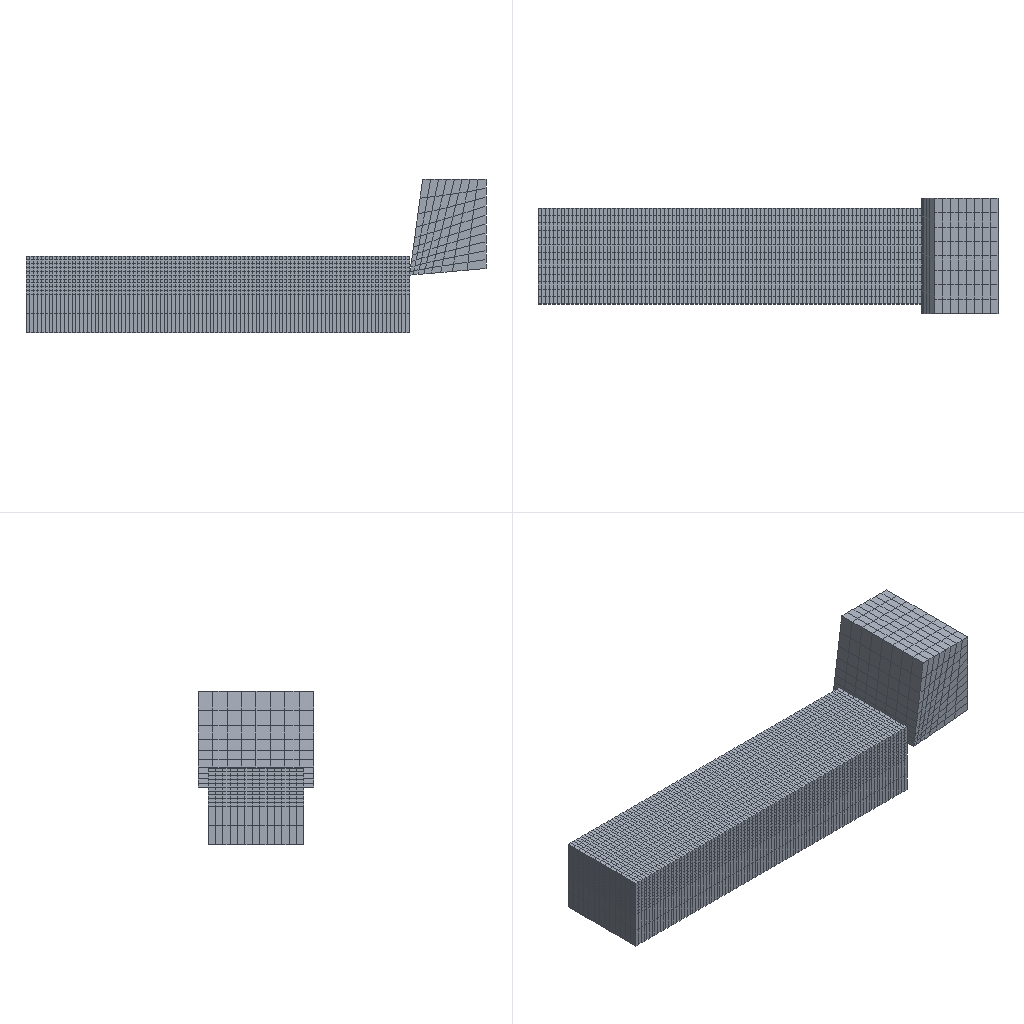Simulation study | abaqus
Set-up summary:
category,name,step,type,value,unit,region
solver,abaqus
solver,version,,,Abaqus/Explicit 2020
units,not stated in the deck,,not stated
analysis,deck,,transient,transient
load_step,Step-1,Step-1,transient
load_step,requested,,,1
mesh,nodes,,,19274
mesh,elements,,,16240
element_type,C3D8R,,solid,16240
load,load commands in deck,,count,1
bc,support commands in deck,,count,7
material,S20MNCR5,,in results
material,S45,,in results
material,TOOL,,in results
check,setup vs results,,match,"per instance, exact: element labels, types and connectivity; labels of the nodes the elements use; coordinates of those nodes at SINGLE_PRECISION in 2 of 2 instance(s)"
Abaqus input file, long lists of numbers shortened:
*Heading
** Job name: Job-1 Model name: Model-1
** Generated by: Abaqus/CAE 2020
*Preprint, echo=NO, model=NO, history=NO, contact=NO
**
** PARTS
**
*Part, name=tool
*Node
      1,  0.7735,          0.5,  0.6
      2,  0.7735,  0.4535,  0.6
** (889 more lines like these left out)
*Element, type=C3D8R
  1, 100, 101, 112, 111,   1,   2,  13,  12
  2, 101, 102, 113, 112,   2,   3,  14,  13
** (638 more lines like these left out)
*Node
    892,  0.7735,          0.5,  0.3
*Nset, nset=tool-RefPt_, internal
892,
*Nset, nset=Set-9, generate
   1,  891,    1
*Elset, elset=Set-9, generate
   1,  640,    1
** Section: tool
*Solid Section, elset=Set-9, material=tool
,
*End Part
**
*Part, name=work
*Node
      1,           0.,           0.,  0.2
      2,           0.,         -0.5,  0.2
** (18380 more lines like these left out)
*Element, type=C3D8R
   1,   278,  1829,  7691,  1037,     1,    17,   941,    48
   2,  1829,  1830,  7692,  7691,    17,    18,   942,   941
** (15598 more lines like these left out)
*Nset, nset=Set-7
     1,     2,     3,     4,     5,     6,     7,     8,    13,    14,    15,    16,    17,    18,    19,    20
    21,    22,    23,    24,    25,    26,    27,    28,    29,    30,    31,    32,    33,    34,    35,    36
** (971 more lines like these left out)
*Elset, elset=Set-7
     1,     2,     3,     4,     5,     6,     7,     8,     9,    10,    11,    12,    13,    14,    15,    16
    17,    18,    19,    20,    21,    22,    23,    24,    25,    26,    27,    28,    29,    30,    31,    32
** (811 more lines like these left out)
*Nset, nset=Set-9
     3,     4,     6,     7,    13,    14,    15,    16,    33,    34,    35,    36,    37,    38,    39,    40
    41,    42,    43,    44,    65,    66,    67,    68,    69,    70,    71,    72,    73,    74,    75,    76
** (529 more lines like these left out)
*Elset, elset=Set-9, generate
  9101,  15600,      1
*Nset, nset=Set-10
     3,     4,     6,     7,    13,    14,    15,    16,    33,    34,    35,    36,    37,    38,    39,    40
    41,    42,    43,    44,    65,    66,    67,    68,    69,    70,    71,    72,    73,    74,    75,    76
** (529 more lines like these left out)
*Elset, elset=Set-10, generate
  9101,  15600,      1
*Nset, nset=Set-11, generate
     1,  18382,      1
*Elset, elset=Set-11, generate
     1,  15600,      1
** Section: work
*Solid Section, elset=Set-11, material=s20mncr5
,
*End Part
**
**
** ASSEMBLY
**
*Assembly, name=Assembly
**
*Instance, name=tool-1, part=tool
       1.625,         0.05,          0.3
       1.625,         0.05,          0.3, 2.625,         0.05,          0.3, 90.
*End Instance
**
*Instance, name=work-1, part=work
*End Instance
**
*Nset, nset=Set-1, instance=work-1
    9,   10,   11,   12,  478,  479,  480,  481,  482,  483,  484,  485,  486,  487,  488,  489
  492,  493,  494,  495,  496,  497,  498,  499,  500,  501,  502,  503,  505,  506,  507,  508
** (87 more lines like these left out)
*Elset, elset=Set-1, instance=work-1
 6514, 6515, 6516, 6517, 6518, 6519, 6520, 6521, 6522, 6523, 6524, 6525, 6526, 6540, 6541, 6542
 6543, 6544, 6545, 6546, 6547, 6548, 6549, 6550, 6551, 6552, 6566, 6567, 6568, 6569, 6570, 6571
** (80 more lines like these left out)
*Nset, nset=Set-2, instance=tool-1
 892,
*Nset, nset=Set-4, instance=tool-1, generate
   1,  891,    1
*Nset, nset=Set-4, instance=work-1
     1,     2,     3,     4,     5,     6,     7,     8,     9,    10,    11,    12,    13,    14,    15,    16
    17,    18,    19,    20,    21,    22,    23,    24,    25,    26,    27,    28,    29,    30,    31,    32
** (1059 more lines like these left out)
*Elset, elset=Set-4, instance=tool-1, generate
   1,  640,    1
*Elset, elset=Set-4, instance=work-1, generate
     1,  15600,      1
*Nset, nset=Set-12, instance=work-1
    9,   10,   11,   12,  478,  479,  480,  481,  482,  483,  484,  485,  486,  487,  488,  489
  492,  493,  494,  495,  496,  497,  498,  499,  500,  501,  502,  503,  505,  506,  507,  508
** (87 more lines like these left out)
*Elset, elset=Set-12, instance=work-1
 6514, 6515, 6516, 6517, 6518, 6519, 6520, 6521, 6522, 6523, 6524, 6525, 6526, 6540, 6541, 6542
 6543, 6544, 6545, 6546, 6547, 6548, 6549, 6550, 6551, 6552, 6566, 6567, 6568, 6569, 6570, 6571
** (80 more lines like these left out)
*Nset, nset=b_Set-5, instance=tool-1, generate
   1,  891,    1
*Elset, elset=b_Set-5, instance=tool-1, generate
   1,  640,    1
*Nset, nset=s_Set-9, instance=work-1
     3,     4,     6,     7,    13,    14,    15,    16,    33,    34,    35,    36,    37,    38,    39,    40
    41,    42,    43,    44,    65,    66,    67,    68,    69,    70,    71,    72,    73,    74,    75,    76
** (529 more lines like these left out)
*Elset, elset=s_Set-9, instance=work-1, generate
  9101,  15600,      1
*Nset, nset=s_Set-10, instance=work-1
     1,     2,     3,     4,     5,     6,     7,     8,    13,    14,    15,    16,    17,    18,    19,    20
    21,    22,    23,    24,    25,    26,    27,    28,    29,    30,    31,    32,    33,    34,    35,    36
** (971 more lines like these left out)
*Elset, elset=s_Set-10, instance=work-1
     1,     2,     3,     4,     5,     6,     7,     8,     9,    10,    11,    12,    13,    14,    15,    16
    17,    18,    19,    20,    21,    22,    23,    24,    25,    26,    27,    28,    29,    30,    31,    32
** (892 more lines like these left out)
*Nset, nset=s_Set-11, instance=work-1
     1,     2,     3,     4,     5,     6,     7,     8,    13,    14,    15,    16,    17,    18,    19,    20
    21,    22,    23,    24,    25,    26,    27,    28,    29,    30,    31,    32,    33,    34,    35,    36
** (971 more lines like these left out)
*Elset, elset=s_Set-11, instance=work-1
     1,     2,     3,     4,     5,     6,     7,     8,     9,    10,    11,    12,    13,    14,    15,    16
    17,    18,    19,    20,    21,    22,    23,    24,    25,    26,    27,    28,    29,    30,    31,    32
** (811 more lines like these left out)
*Nset, nset=_PickedSet13, internal, instance=tool-1
 892,
*Elset, elset=_Surf-4_S5, internal, instance=work-1
  9153,  9154,  9155,  9156,  9157,  9158,  9159,  9160,  9161,  9162,  9163,  9164,  9165,  9218,  9219,  9220
  9221,  9222,  9223,  9224,  9225,  9226,  9227,  9228,  9229,  9230,  9283,  9284,  9285,  9286,  9287,  9288
** (80 more lines like these left out)
*Surface, type=ELEMENT, name=Surf-4
_Surf-4_S5, S5
*Elset, elset=_m_Surf-1_S1, internal, instance=tool-1, generate
 561,  640,    1
*Elset, elset=_m_Surf-1_S6, internal, instance=tool-1, generate
   1,  631,   10
*Elset, elset=_m_Surf-1_S2, internal, instance=tool-1, generate
  1,  80,   1
*Elset, elset=_m_Surf-1_S4, internal, instance=tool-1, generate
  10,  640,   10
*Elset, elset=_m_Surf-1_S3, internal, instance=tool-1
   1,   2,   3,   4,   5,   6,   7,   8,   9,  10,  81,  82,  83,  84,  85,  86
  87,  88,  89,  90, 161, 162, 163, 164, 165, 166, 167, 168, 169, 170, 241, 242
** (3 more lines like these left out)
*Elset, elset=_m_Surf-1_S5, internal, instance=tool-1
  71,  72,  73,  74,  75,  76,  77,  78,  79,  80, 151, 152, 153, 154, 155, 156
 157, 158, 159, 160, 231, 232, 233, 234, 235, 236, 237, 238, 239, 240, 311, 312
** (3 more lines like these left out)
*Surface, type=ELEMENT, name=m_Surf-1
_m_Surf-1_S1, S1
_m_Surf-1_S6, S6
_m_Surf-1_S2, S2
_m_Surf-1_S4, S4
_m_Surf-1_S3, S3
_m_Surf-1_S5, S5
*Elset, elset=_m_Surf-3_S1, internal, instance=tool-1, generate
 561,  640,    1
*Elset, elset=_m_Surf-3_S6, internal, instance=tool-1, generate
   1,  631,   10
*Elset, elset=_m_Surf-3_S2, internal, instance=tool-1, generate
  1,  80,   1
*Elset, elset=_m_Surf-3_S4, internal, instance=tool-1, generate
  10,  640,   10
*Elset, elset=_m_Surf-3_S3, internal, instance=tool-1
   1,   2,   3,   4,   5,   6,   7,   8,   9,  10,  81,  82,  83,  84,  85,  86
  87,  88,  89,  90, 161, 162, 163, 164, 165, 166, 167, 168, 169, 170, 241, 242
** (3 more lines like these left out)
*Elset, elset=_m_Surf-3_S5, internal, instance=tool-1
  71,  72,  73,  74,  75,  76,  77,  78,  79,  80, 151, 152, 153, 154, 155, 156
 157, 158, 159, 160, 231, 232, 233, 234, 235, 236, 237, 238, 239, 240, 311, 312
** (3 more lines like these left out)
*Surface, type=ELEMENT, name=m_Surf-3
_m_Surf-3_S1, S1
_m_Surf-3_S6, S6
_m_Surf-3_S2, S2
_m_Surf-3_S4, S4
_m_Surf-3_S3, S3
_m_Surf-3_S5, S5
*Surface, type=NODE, name=s_Set-11_CNS_, internal
s_Set-11, 1.
** Constraint: Constraint-1
*Rigid Body, ref node=_PickedSet13, elset=b_Set-5
*End Assembly
**
** MATERIALS
**
*Material, name=s20mncr5
*Damage Initiation, criterion=SHEAR
1.,0.,0.
*Damage Evolution, type=DISPLACEMENT
 0.001,
*Density
 8.24e-09,
*Elastic
200000., 0.3
*Expansion
 1.3e-05,
*Plastic
1200.,0.
*Material, name=s45
*Conductivity
 50.2,
*Density
 7.8e-09,
*Elastic
210000., 0.3
*Expansion
 1.5e-05,
*Plastic, hardening=JOHNSON COOK
507., 320., 0.28, 1.06,1538.,  25.
*Rate Dependent, type=JOHNSON COOK
 0.064,1.
*Specific Heat
 5e+08,
*Material, name=tool
*Conductivity
120.,
*Density
 1.57e-08,
*Elastic
650000., 0.22
*Expansion
 5.2e-06,
*Specific Heat
 3.43e+08,
**
** INTERACTION PROPERTIES
**
*Surface Interaction, name=IntProp-1
*Friction
 0.2,
*Surface Behavior, pressure-overclosure=HARD
*Surface Interaction, name=chip
*Friction
 0.5,
*Surface Behavior, pressure-overclosure=HARD
**
** BOUNDARY CONDITIONS
**
** Name: BC-1 Type: 对称/反对称/完全固定
*Boundary
Set-12, ENCASTRE
** ----------------------------------------------------------------
**
** STEP: Step-1
**
*Step, name=Step-1, nlgeom=YES
*Dynamic, Explicit
, 0.0014
*Bulk Viscosity
0.06, 1.2
** Mass Scaling: Semi-Automatic
**               Whole Model
*Fixed Mass Scaling, factor=50.
**
** BOUNDARY CONDITIONS
**
** Name: [REDACTED] : Velocity/Angular velocity
*Boundary, type=VELOCITY
Set-2, 1, 1, -2000.
Set-2, 2, 2
Set-2, 3, 3
Set-2, 4, 4
Set-2, 5, 5
Set-2, 6, 6
**
** INTERACTIONS
**
** Interaction: Int-1
*Contact Pair, interaction=IntProp-1, mechanical constraint=KINEMATIC, cpset=Int-1
m_Surf-3, s_Set-11_CNS_
** Interaction: Int-2
*Contact Pair, interaction=chip, mechanical constraint=KINEMATIC, cpset=Int-2
Surf-4,
**
** OUTPUT REQUESTS
**
*Restart, write, number interval=1, time marks=NO
**
** FIELD OUTPUT: F-Output-1
**
*Output, field, number interval=100
*Node Output
A, CF, RF, RM, RT, U, V
*Element Output, directions=YES
E, EVF, LE, MISES, MISESMAX, PE, PEEQ, PEEQMAX, PEEQT, PEEQVAVG, PEMAG, PEVAVG, S, SF, STATUS, SVAVG
*Contact Output
CDISP, CSTRESS
**
** HISTORY OUTPUT: H-Output-1
**
*Output, history, time interval=4.66667e-07
*Node Output, nset=Set-2
RF1, RF2, RF3
*End Step
Results summary:
result,step,Step-1,partial,increments=74724 time=0.000842/0.0014
result,analysis,,,transient
result,last_loadstep,,,1
result,primary field,,,U
result,reaction total,,FX,37.455,model units
result,reaction total,,FY,-8.456,model units
result,reaction total,,FZ,29.936,model units